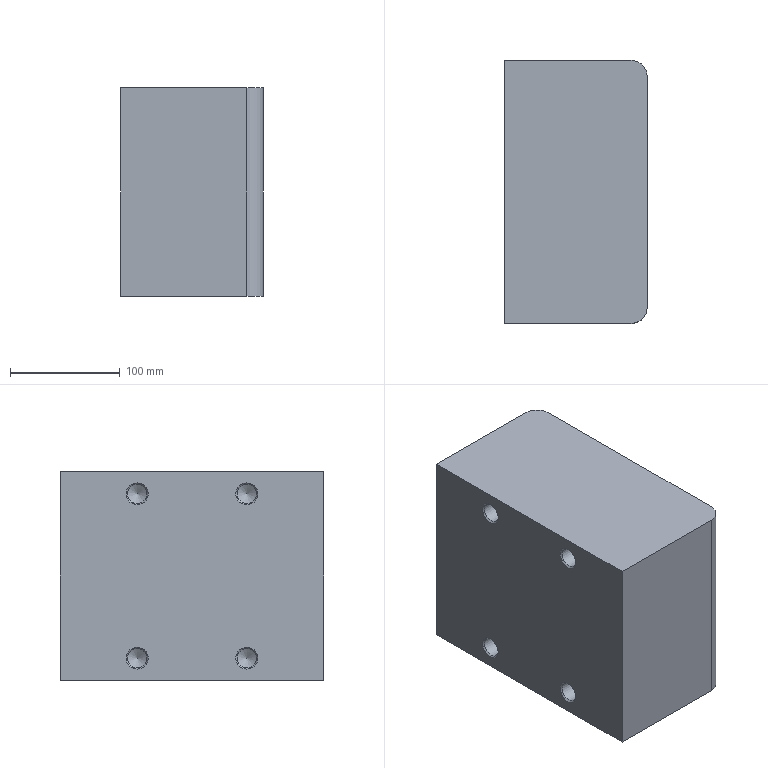Part | NX | features SIMPLE HOLE 4, SYMBOLIC_THREAD 4, DATUM_CSYS 3, SKETCH 2, BLEND 1, EXTRUDE 1, HOLE PACKAGE 1 | 1 solid | 20 faces | box 130 x 240 x 190.5 mm | volume 5884853 mm3 | cone 8 | plane 6 | cylinder 6 | commonest cylinder face diameters 17.5 x4 30 x2
STEP:
#1=CARTESIAN_POINT('',(115.,-120.,-95.25));
#2=VERTEX_POINT('',#1);
#3=CARTESIAN_POINT('',(0.,-120.,-95.25));
#4=VERTEX_POINT('',#3);
#5=CARTESIAN_POINT('',(130.,-120.,-95.25));
#6=DIRECTION('',(-1.,0.,0.));
#7=VECTOR('',#6,1000.);
#8=LINE('',#5,#7);
#9=EDGE_CURVE('',#2,#4,#8,.T.);
#10=ORIENTED_EDGE('',*,*,#9,.F.);
#11=CARTESIAN_POINT('',(115.,-120.,95.25));
#12=VERTEX_POINT('',#11);
#13=CARTESIAN_POINT('',(115.,-120.,95.25));
#14=DIRECTION('',(0.,0.,-1.));
#15=VECTOR('',#14,1000.);
#16=LINE('',#13,#15);
#17=EDGE_CURVE('',#2,#12,#16,.F.);
#18=ORIENTED_EDGE('',*,*,#17,.T.);
#19=CARTESIAN_POINT('',(0.,-120.,95.25));
#20=VERTEX_POINT('',#19);
#21=CARTESIAN_POINT('',(130.,-120.,95.25));
#22=DIRECTION('',(-1.,0.,0.));
#23=VECTOR('',#22,1000.);
#24=LINE('',#21,#23);
#25=EDGE_CURVE('',#12,#20,#24,.T.);
#26=ORIENTED_EDGE('',*,*,#25,.T.);
#27=CARTESIAN_POINT('',(0.,-120.,95.25));
#28=DIRECTION('',(0.,0.,-1.));
#29=VECTOR('',#28,1000.);
#30=LINE('',#27,#29);
#31=EDGE_CURVE('',#20,#4,#30,.T.);
#32=ORIENTED_EDGE('',*,*,#31,.T.);
#33=EDGE_LOOP('',(#10,#18,#26,#32));
#34=FACE_BOUND('',#33,.T.);
#35=CARTESIAN_POINT('',(130.,-120.,95.25));
#36=DIRECTION('',(0.,1.,0.));
#37=DIRECTION('',(0.,0.,1.));
#38=AXIS2_PLACEMENT_3D('',#35,#36,#37);
#39=PLANE('',#38);
#40=ADVANCED_FACE('',(#34),#39,.F.);
#41=CARTESIAN_POINT('',(130.,-105.,-95.25));
#42=VERTEX_POINT('',#41);
#43=CARTESIAN_POINT('',(130.,105.,-95.25));
#44=VERTEX_POINT('',#43);
#45=CARTESIAN_POINT('',(130.,-120.,-95.25));
#46=DIRECTION('',(0.,1.,0.));
#47=VECTOR('',#46,1000.);
#48=LINE('',#45,#47);
#49=EDGE_CURVE('',#42,#44,#48,.T.);
#50=ORIENTED_EDGE('',*,*,#49,.F.);
#51=CARTESIAN_POINT('',(115.,-105.,-95.25));
#52=DIRECTION('',(0.,0.,1.));
#53=DIRECTION('',(1.,0.,0.));
#54=AXIS2_PLACEMENT_3D('',#51,#52,#53);
#55=CIRCLE('',#54,15.);
#56=EDGE_CURVE('',#42,#2,#55,.F.);
#57=ORIENTED_EDGE('',*,*,#56,.T.);
#58=ORIENTED_EDGE('',*,*,#9,.T.);
#59=CARTESIAN_POINT('',(0.,120.,-95.25));
#60=VERTEX_POINT('',#59);
#61=CARTESIAN_POINT('',(0.,-120.,-95.25));
#62=DIRECTION('',(0.,1.,0.));
#63=VECTOR('',#62,1000.);
#64=LINE('',#61,#63);
#65=EDGE_CURVE('',#4,#60,#64,.T.);
#66=ORIENTED_EDGE('',*,*,#65,.T.);
#67=CARTESIAN_POINT('',(115.,120.,-95.25));
#68=VERTEX_POINT('',#67);
#69=CARTESIAN_POINT('',(130.,120.,-95.25));
#70=DIRECTION('',(-1.,0.,0.));
#71=VECTOR('',#70,1000.);
#72=LINE('',#69,#71);
#73=EDGE_CURVE('',#68,#60,#72,.T.);
#74=ORIENTED_EDGE('',*,*,#73,.F.);
#75=CARTESIAN_POINT('',(115.,105.,-95.25));
#76=DIRECTION('',(0.,0.,1.));
#77=DIRECTION('',(1.,0.,0.));
#78=AXIS2_PLACEMENT_3D('',#75,#76,#77);
#79=CIRCLE('',#78,15.);
#80=EDGE_CURVE('',#68,#44,#79,.F.);
#81=ORIENTED_EDGE('',*,*,#80,.T.);
#82=EDGE_LOOP('',(#50,#57,#58,#66,#74,#81));
#83=FACE_BOUND('',#82,.T.);
#84=CARTESIAN_POINT('',(130.,-120.,-95.25));
#85=DIRECTION('',(0.,0.,1.));
#86=DIRECTION('',(1.,0.,0.));
#87=AXIS2_PLACEMENT_3D('',#84,#85,#86);
#88=PLANE('',#87);
#89=ADVANCED_FACE('',(#83),#88,.F.);
#90=CARTESIAN_POINT('',(115.,120.,95.25));
#91=VERTEX_POINT('',#90);
#92=CARTESIAN_POINT('',(0.,120.,95.25));
#93=VERTEX_POINT('',#92);
#94=CARTESIAN_POINT('',(130.,120.,95.25));
#95=DIRECTION('',(-1.,0.,0.));
#96=VECTOR('',#95,1000.);
#97=LINE('',#94,#96);
#98=EDGE_CURVE('',#91,#93,#97,.T.);
#99=ORIENTED_EDGE('',*,*,#98,.F.);
#100=CARTESIAN_POINT('',(115.,120.,-95.25));
#101=DIRECTION('',(0.,0.,1.));
#102=VECTOR('',#101,1000.);
#103=LINE('',#100,#102);
#104=EDGE_CURVE('',#91,#68,#103,.F.);
#105=ORIENTED_EDGE('',*,*,#104,.T.);
#106=ORIENTED_EDGE('',*,*,#73,.T.);
#107=CARTESIAN_POINT('',(0.,120.,-95.25));
#108=DIRECTION('',(0.,0.,1.));
#109=VECTOR('',#108,1000.);
#110=LINE('',#107,#109);
#111=EDGE_CURVE('',#60,#93,#110,.T.);
#112=ORIENTED_EDGE('',*,*,#111,.T.);
#113=EDGE_LOOP('',(#99,#105,#106,#112));
#114=FACE_BOUND('',#113,.T.);
#115=CARTESIAN_POINT('',(130.,120.,-95.25));
#116=DIRECTION('',(0.,-1.,0.));
#117=DIRECTION('',(0.,0.,-1.));
#118=AXIS2_PLACEMENT_3D('',#115,#116,#117);
#119=PLANE('',#118);
#120=ADVANCED_FACE('',(#114),#119,.F.);
#121=ORIENTED_EDGE('',*,*,#25,.F.);
#122=CARTESIAN_POINT('',(130.,-105.,95.25));
#123=VERTEX_POINT('',#122);
#124=CARTESIAN_POINT('',(115.,-105.,95.25));
#125=DIRECTION('',(0.,0.,-1.));
#126=DIRECTION('',(-1.,0.,0.));
#127=AXIS2_PLACEMENT_3D('',#124,#125,#126);
#128=CIRCLE('',#127,15.);
#129=EDGE_CURVE('',#12,#123,#128,.F.);
#130=ORIENTED_EDGE('',*,*,#129,.T.);
#131=CARTESIAN_POINT('',(130.,105.,95.25));
#132=VERTEX_POINT('',#131);
#133=CARTESIAN_POINT('',(130.,120.,95.25));
#134=DIRECTION('',(0.,-1.,0.));
#135=VECTOR('',#134,1000.);
#136=LINE('',#133,#135);
#137=EDGE_CURVE('',#132,#123,#136,.T.);
#138=ORIENTED_EDGE('',*,*,#137,.F.);
#139=CARTESIAN_POINT('',(115.,105.,95.25));
#140=DIRECTION('',(0.,0.,-1.));
#141=DIRECTION('',(-1.,0.,0.));
#142=AXIS2_PLACEMENT_3D('',#139,#140,#141);
#143=CIRCLE('',#142,15.);
#144=EDGE_CURVE('',#132,#91,#143,.F.);
#145=ORIENTED_EDGE('',*,*,#144,.T.);
#146=ORIENTED_EDGE('',*,*,#98,.T.);
#147=CARTESIAN_POINT('',(0.,120.,95.25));
#148=DIRECTION('',(0.,-1.,0.));
#149=VECTOR('',#148,1000.);
#150=LINE('',#147,#149);
#151=EDGE_CURVE('',#93,#20,#150,.T.);
#152=ORIENTED_EDGE('',*,*,#151,.T.);
#153=EDGE_LOOP('',(#121,#130,#138,#145,#146,#152));
#154=FACE_BOUND('',#153,.T.);
#155=CARTESIAN_POINT('',(130.,120.,95.25));
#156=DIRECTION('',(0.,0.,-1.));
#157=DIRECTION('',(-1.,0.,0.));
#158=AXIS2_PLACEMENT_3D('',#155,#156,#157);
#159=PLANE('',#158);
#160=ADVANCED_FACE('',(#154),#159,.F.);
#161=ORIENTED_EDGE('',*,*,#137,.T.);
#162=CARTESIAN_POINT('',(130.,-105.,-95.25));
#163=DIRECTION('',(0.,0.,-1.));
#164=VECTOR('',#163,1000.);
#165=LINE('',#162,#164);
#166=EDGE_CURVE('',#123,#42,#165,.T.);
#167=ORIENTED_EDGE('',*,*,#166,.T.);
#168=ORIENTED_EDGE('',*,*,#49,.T.);
#169=CARTESIAN_POINT('',(130.,105.,95.25));
#170=DIRECTION('',(0.,0.,1.));
#171=VECTOR('',#170,1000.);
#172=LINE('',#169,#171);
#173=EDGE_CURVE('',#44,#132,#172,.T.);
#174=ORIENTED_EDGE('',*,*,#173,.T.);
#175=EDGE_LOOP('',(#161,#167,#168,#174));
#176=FACE_BOUND('',#175,.T.);
#177=CARTESIAN_POINT('',(130.,0.,0.));
#178=DIRECTION('',(1.,0.,0.));
#179=DIRECTION('',(0.,0.,-1.));
#180=AXIS2_PLACEMENT_3D('',#177,#178,#179);
#181=PLANE('',#180);
#182=ADVANCED_FACE('',(#176),#181,.T.);
#183=CARTESIAN_POINT('',(0.,50.,65.));
#184=VERTEX_POINT('',#183);
#185=CARTESIAN_POINT('',(0.,50.,75.));
#186=DIRECTION('',(1.,0.,0.));
#187=DIRECTION('',(0.,0.,-1.));
#188=AXIS2_PLACEMENT_3D('',#185,#186,#187);
#189=CIRCLE('',#188,10.);
#190=EDGE_CURVE('',#184,#184,#189,.T.);
#191=ORIENTED_EDGE('',*,*,#190,.T.);
#192=EDGE_LOOP('',(#191));
#193=FACE_BOUND('',#192,.T.);
#194=CARTESIAN_POINT('',(0.,50.,-85.));
#195=VERTEX_POINT('',#194);
#196=CARTESIAN_POINT('',(0.,50.,-75.));
#197=DIRECTION('',(1.,0.,0.));
#198=DIRECTION('',(0.,0.,-1.));
#199=AXIS2_PLACEMENT_3D('',#196,#197,#198);
#200=CIRCLE('',#199,10.);
#201=EDGE_CURVE('',#195,#195,#200,.T.);
#202=ORIENTED_EDGE('',*,*,#201,.T.);
#203=EDGE_LOOP('',(#202));
#204=FACE_BOUND('',#203,.T.);
#205=CARTESIAN_POINT('',(0.,-50.,65.));
#206=VERTEX_POINT('',#205);
#207=CARTESIAN_POINT('',(0.,-50.,75.));
#208=DIRECTION('',(1.,0.,0.));
#209=DIRECTION('',(0.,0.,-1.));
#210=AXIS2_PLACEMENT_3D('',#207,#208,#209);
#211=CIRCLE('',#210,10.);
#212=EDGE_CURVE('',#206,#206,#211,.T.);
#213=ORIENTED_EDGE('',*,*,#212,.T.);
#214=EDGE_LOOP('',(#213));
#215=FACE_BOUND('',#214,.T.);
#216=CARTESIAN_POINT('',(0.,-50.,-85.));
#217=VERTEX_POINT('',#216);
#218=CARTESIAN_POINT('',(0.,-50.,-75.));
#219=DIRECTION('',(1.,0.,0.));
#220=DIRECTION('',(0.,0.,-1.));
#221=AXIS2_PLACEMENT_3D('',#218,#219,#220);
#222=CIRCLE('',#221,10.);
#223=EDGE_CURVE('',#217,#217,#222,.T.);
#224=ORIENTED_EDGE('',*,*,#223,.T.);
#225=EDGE_LOOP('',(#224));
#226=FACE_BOUND('',#225,.T.);
#227=ORIENTED_EDGE('',*,*,#31,.F.);
#228=ORIENTED_EDGE('',*,*,#151,.F.);
#229=ORIENTED_EDGE('',*,*,#111,.F.);
#230=ORIENTED_EDGE('',*,*,#65,.F.);
#231=EDGE_LOOP('',(#227,#228,#229,#230));
#232=FACE_BOUND('',#231,.T.);
#233=CARTESIAN_POINT('',(0.,0.,0.));
#234=DIRECTION('',(1.,0.,0.));
#235=DIRECTION('',(0.,0.,-1.));
#236=AXIS2_PLACEMENT_3D('',#233,#234,#235);
#237=PLANE('',#236);
#238=ADVANCED_FACE('',(#193,#204,#215,#226,#232),#237,.F.);
#239=ORIENTED_EDGE('',*,*,#129,.F.);
#240=ORIENTED_EDGE('',*,*,#17,.F.);
#241=ORIENTED_EDGE('',*,*,#56,.F.);
#242=ORIENTED_EDGE('',*,*,#166,.F.);
#243=EDGE_LOOP('',(#239,#240,#241,#242));
#244=FACE_BOUND('',#243,.T.);
#245=CARTESIAN_POINT('',(115.,-105.,0.));
#246=DIRECTION('',(0.,0.,1.));
#247=DIRECTION('',(1.,0.,0.));
#248=AXIS2_PLACEMENT_3D('',#245,#246,#247);
#249=CYLINDRICAL_SURFACE('',#248,15.);
#250=ADVANCED_FACE('',(#244),#249,.T.);
#251=ORIENTED_EDGE('',*,*,#80,.F.);
#252=ORIENTED_EDGE('',*,*,#104,.F.);
#253=ORIENTED_EDGE('',*,*,#144,.F.);
#254=ORIENTED_EDGE('',*,*,#173,.F.);
#255=EDGE_LOOP('',(#251,#252,#253,#254));
#256=FACE_BOUND('',#255,.T.);
#257=CARTESIAN_POINT('',(115.,105.,0.));
#258=DIRECTION('',(0.,0.,-1.));
#259=DIRECTION('',(-1.,0.,0.));
#260=AXIS2_PLACEMENT_3D('',#257,#258,#259);
#261=CYLINDRICAL_SURFACE('',#260,15.);
#262=ADVANCED_FACE('',(#256),#261,.T.);
#263=CARTESIAN_POINT('',(40.,-50.,-83.75));
#264=VERTEX_POINT('',#263);
#265=CARTESIAN_POINT('',(40.,-50.,-75.));
#266=DIRECTION('',(1.,0.,0.));
#267=DIRECTION('',(0.,0.,-1.));
#268=AXIS2_PLACEMENT_3D('',#265,#266,#267);
#269=CIRCLE('',#268,8.75);
#270=EDGE_CURVE('',#264,#264,#269,.F.);
#271=ORIENTED_EDGE('',*,*,#270,.T.);
#272=EDGE_LOOP('',(#271));
#273=FACE_BOUND('',#272,.T.);
#274=CARTESIAN_POINT('',(45.258,-50.,-75.));
#275=VERTEX_POINT('',#274);
#276=VERTEX_LOOP('',#275);
#277=FACE_BOUND('',#276,.T.);
#278=CARTESIAN_POINT('',(40.,-50.,-75.));
#279=DIRECTION('',(-1.,0.,0.));
#280=DIRECTION('',(0.,0.,1.));
#281=AXIS2_PLACEMENT_3D('',#278,#279,#280);
#282=CONICAL_SURFACE('',#281,8.75,1.03);
#283=ADVANCED_FACE('',(#273,#277),#282,.F.);
#284=CARTESIAN_POINT('',(1.25,-50.,-83.75));
#285=VERTEX_POINT('',#284);
#286=CARTESIAN_POINT('',(1.25,-50.,-75.));
#287=DIRECTION('',(1.,0.,0.));
#288=DIRECTION('',(0.,0.,-1.));
#289=AXIS2_PLACEMENT_3D('',#286,#287,#288);
#290=CIRCLE('',#289,8.75);
#291=EDGE_CURVE('',#285,#285,#290,.F.);
#292=ORIENTED_EDGE('',*,*,#291,.T.);
#293=EDGE_LOOP('',(#292));
#294=FACE_BOUND('',#293,.T.);
#295=ORIENTED_EDGE('',*,*,#270,.F.);
#296=EDGE_LOOP('',(#295));
#297=FACE_BOUND('',#296,.T.);
#298=CARTESIAN_POINT('',(0.,-50.,-75.));
#299=DIRECTION('',(1.,0.,0.));
#300=DIRECTION('',(0.,0.,-1.));
#301=AXIS2_PLACEMENT_3D('',#298,#299,#300);
#302=CYLINDRICAL_SURFACE('',#301,8.75);
#303=ADVANCED_FACE('',(#294,#297),#302,.F.);
#304=ORIENTED_EDGE('',*,*,#291,.F.);
#305=EDGE_LOOP('',(#304));
#306=FACE_BOUND('',#305,.T.);
#307=ORIENTED_EDGE('',*,*,#223,.F.);
#308=EDGE_LOOP('',(#307));
#309=FACE_BOUND('',#308,.T.);
#310=CARTESIAN_POINT('',(0.,-50.,-75.));
#311=DIRECTION('',(-1.,0.,0.));
#312=DIRECTION('',(0.,0.,1.));
#313=AXIS2_PLACEMENT_3D('',#310,#311,#312);
#314=CONICAL_SURFACE('',#313,10.,0.7854);
#315=ADVANCED_FACE('',(#306,#309),#314,.F.);
#316=CARTESIAN_POINT('',(40.,-50.,66.25));
#317=VERTEX_POINT('',#316);
#318=CARTESIAN_POINT('',(40.,-50.,75.));
#319=DIRECTION('',(1.,0.,0.));
#320=DIRECTION('',(0.,0.,-1.));
#321=AXIS2_PLACEMENT_3D('',#318,#319,#320);
#322=CIRCLE('',#321,8.75);
#323=EDGE_CURVE('',#317,#317,#322,.F.);
#324=ORIENTED_EDGE('',*,*,#323,.T.);
#325=EDGE_LOOP('',(#324));
#326=FACE_BOUND('',#325,.T.);
#327=CARTESIAN_POINT('',(45.258,-50.,75.));
#328=VERTEX_POINT('',#327);
#329=VERTEX_LOOP('',#328);
#330=FACE_BOUND('',#329,.T.);
#331=CARTESIAN_POINT('',(40.,-50.,75.));
#332=DIRECTION('',(-1.,0.,0.));
#333=DIRECTION('',(0.,0.,1.));
#334=AXIS2_PLACEMENT_3D('',#331,#332,#333);
#335=CONICAL_SURFACE('',#334,8.75,1.03);
#336=ADVANCED_FACE('',(#326,#330),#335,.F.);
#337=CARTESIAN_POINT('',(1.25,-50.,66.25));
#338=VERTEX_POINT('',#337);
#339=CARTESIAN_POINT('',(1.25,-50.,75.));
#340=DIRECTION('',(1.,0.,0.));
#341=DIRECTION('',(0.,0.,-1.));
#342=AXIS2_PLACEMENT_3D('',#339,#340,#341);
#343=CIRCLE('',#342,8.75);
#344=EDGE_CURVE('',#338,#338,#343,.F.);
#345=ORIENTED_EDGE('',*,*,#344,.T.);
#346=EDGE_LOOP('',(#345));
#347=FACE_BOUND('',#346,.T.);
#348=ORIENTED_EDGE('',*,*,#323,.F.);
#349=EDGE_LOOP('',(#348));
#350=FACE_BOUND('',#349,.T.);
#351=CARTESIAN_POINT('',(0.,-50.,75.));
#352=DIRECTION('',(1.,0.,0.));
#353=DIRECTION('',(0.,0.,-1.));
#354=AXIS2_PLACEMENT_3D('',#351,#352,#353);
#355=CYLINDRICAL_SURFACE('',#354,8.75);
#356=ADVANCED_FACE('',(#347,#350),#355,.F.);
#357=ORIENTED_EDGE('',*,*,#344,.F.);
#358=EDGE_LOOP('',(#357));
#359=FACE_BOUND('',#358,.T.);
#360=ORIENTED_EDGE('',*,*,#212,.F.);
#361=EDGE_LOOP('',(#360));
#362=FACE_BOUND('',#361,.T.);
#363=CARTESIAN_POINT('',(0.,-50.,75.));
#364=DIRECTION('',(-1.,0.,0.));
#365=DIRECTION('',(0.,0.,1.));
#366=AXIS2_PLACEMENT_3D('',#363,#364,#365);
#367=CONICAL_SURFACE('',#366,10.,0.7854);
#368=ADVANCED_FACE('',(#359,#362),#367,.F.);
#369=CARTESIAN_POINT('',(40.,50.,-83.75));
#370=VERTEX_POINT('',#369);
#371=CARTESIAN_POINT('',(40.,50.,-75.));
#372=DIRECTION('',(1.,0.,0.));
#373=DIRECTION('',(0.,0.,-1.));
#374=AXIS2_PLACEMENT_3D('',#371,#372,#373);
#375=CIRCLE('',#374,8.75);
#376=EDGE_CURVE('',#370,#370,#375,.F.);
#377=ORIENTED_EDGE('',*,*,#376,.T.);
#378=EDGE_LOOP('',(#377));
#379=FACE_BOUND('',#378,.T.);
#380=CARTESIAN_POINT('',(45.258,50.,-75.));
#381=VERTEX_POINT('',#380);
#382=VERTEX_LOOP('',#381);
#383=FACE_BOUND('',#382,.T.);
#384=CARTESIAN_POINT('',(40.,50.,-75.));
#385=DIRECTION('',(-1.,0.,0.));
#386=DIRECTION('',(0.,0.,1.));
#387=AXIS2_PLACEMENT_3D('',#384,#385,#386);
#388=CONICAL_SURFACE('',#387,8.75,1.03);
#389=ADVANCED_FACE('',(#379,#383),#388,.F.);
#390=CARTESIAN_POINT('',(1.25,50.,-83.75));
#391=VERTEX_POINT('',#390);
#392=CARTESIAN_POINT('',(1.25,50.,-75.));
#393=DIRECTION('',(1.,0.,0.));
#394=DIRECTION('',(0.,0.,-1.));
#395=AXIS2_PLACEMENT_3D('',#392,#393,#394);
#396=CIRCLE('',#395,8.75);
#397=EDGE_CURVE('',#391,#391,#396,.F.);
#398=ORIENTED_EDGE('',*,*,#397,.T.);
#399=EDGE_LOOP('',(#398));
#400=FACE_BOUND('',#399,.T.);
#401=ORIENTED_EDGE('',*,*,#376,.F.);
#402=EDGE_LOOP('',(#401));
#403=FACE_BOUND('',#402,.T.);
#404=CARTESIAN_POINT('',(0.,50.,-75.));
#405=DIRECTION('',(1.,0.,0.));
#406=DIRECTION('',(0.,0.,-1.));
#407=AXIS2_PLACEMENT_3D('',#404,#405,#406);
#408=CYLINDRICAL_SURFACE('',#407,8.75);
#409=ADVANCED_FACE('',(#400,#403),#408,.F.);
#410=ORIENTED_EDGE('',*,*,#397,.F.);
#411=EDGE_LOOP('',(#410));
#412=FACE_BOUND('',#411,.T.);
#413=ORIENTED_EDGE('',*,*,#201,.F.);
#414=EDGE_LOOP('',(#413));
#415=FACE_BOUND('',#414,.T.);
#416=CARTESIAN_POINT('',(0.,50.,-75.));
#417=DIRECTION('',(-1.,0.,0.));
#418=DIRECTION('',(0.,0.,1.));
#419=AXIS2_PLACEMENT_3D('',#416,#417,#418);
#420=CONICAL_SURFACE('',#419,10.,0.7854);
#421=ADVANCED_FACE('',(#412,#415),#420,.F.);
#422=CARTESIAN_POINT('',(40.,50.,66.25));
#423=VERTEX_POINT('',#422);
#424=CARTESIAN_POINT('',(40.,50.,75.));
#425=DIRECTION('',(1.,0.,0.));
#426=DIRECTION('',(0.,0.,-1.));
#427=AXIS2_PLACEMENT_3D('',#424,#425,#426);
#428=CIRCLE('',#427,8.75);
#429=EDGE_CURVE('',#423,#423,#428,.F.);
#430=ORIENTED_EDGE('',*,*,#429,.T.);
#431=EDGE_LOOP('',(#430));
#432=FACE_BOUND('',#431,.T.);
#433=CARTESIAN_POINT('',(45.258,50.,75.));
#434=VERTEX_POINT('',#433);
#435=VERTEX_LOOP('',#434);
#436=FACE_BOUND('',#435,.T.);
#437=CARTESIAN_POINT('',(40.,50.,75.));
#438=DIRECTION('',(-1.,0.,0.));
#439=DIRECTION('',(0.,0.,1.));
#440=AXIS2_PLACEMENT_3D('',#437,#438,#439);
#441=CONICAL_SURFACE('',#440,8.75,1.03);
#442=ADVANCED_FACE('',(#432,#436),#441,.F.);
#443=CARTESIAN_POINT('',(1.25,50.,66.25));
#444=VERTEX_POINT('',#443);
#445=CARTESIAN_POINT('',(1.25,50.,75.));
#446=DIRECTION('',(1.,0.,0.));
#447=DIRECTION('',(0.,0.,-1.));
#448=AXIS2_PLACEMENT_3D('',#445,#446,#447);
#449=CIRCLE('',#448,8.75);
#450=EDGE_CURVE('',#444,#444,#449,.F.);
#451=ORIENTED_EDGE('',*,*,#450,.T.);
#452=EDGE_LOOP('',(#451));
#453=FACE_BOUND('',#452,.T.);
#454=ORIENTED_EDGE('',*,*,#429,.F.);
#455=EDGE_LOOP('',(#454));
#456=FACE_BOUND('',#455,.T.);
#457=CARTESIAN_POINT('',(0.,50.,75.));
#458=DIRECTION('',(1.,0.,0.));
#459=DIRECTION('',(0.,0.,-1.));
#460=AXIS2_PLACEMENT_3D('',#457,#458,#459);
#461=CYLINDRICAL_SURFACE('',#460,8.75);
#462=ADVANCED_FACE('',(#453,#456),#461,.F.);
#463=ORIENTED_EDGE('',*,*,#450,.F.);
#464=EDGE_LOOP('',(#463));
#465=FACE_BOUND('',#464,.T.);
#466=ORIENTED_EDGE('',*,*,#190,.F.);
#467=EDGE_LOOP('',(#466));
#468=FACE_BOUND('',#467,.T.);
#469=CARTESIAN_POINT('',(0.,50.,75.));
#470=DIRECTION('',(-1.,0.,0.));
#471=DIRECTION('',(0.,0.,1.));
#472=AXIS2_PLACEMENT_3D('',#469,#470,#471);
#473=CONICAL_SURFACE('',#472,10.,0.7854);
#474=ADVANCED_FACE('',(#465,#468),#473,.F.);
#475=CLOSED_SHELL('',(#40,#89,#120,#160,#182,#238,#250,#262,#283,#303,#315,#336,#356,#368,#389,#409,#421,#442,#462,#474));
#476=MANIFOLD_SOLID_BREP('',#475);
#477=(LENGTH_UNIT()NAMED_UNIT(*)SI_UNIT(.MILLI.,.METRE.));
#478=UNCERTAINTY_MEASURE_WITH_UNIT(LENGTH_MEASURE(0.00001),#477,'','');
#479=(NAMED_UNIT(*)PLANE_ANGLE_UNIT()SI_UNIT($,.RADIAN.));
#480=(NAMED_UNIT(*)SI_UNIT($,.STERADIAN.)SOLID_ANGLE_UNIT());
#481=(GEOMETRIC_REPRESENTATION_CONTEXT(3)GLOBAL_UNCERTAINTY_ASSIGNED_CONTEXT((#478))GLOBAL_UNIT_ASSIGNED_CONTEXT((#477,#479,#480))REPRESENTATION_CONTEXT('',''));
#482=ADVANCED_BREP_SHAPE_REPRESENTATION('',(#476),#481);